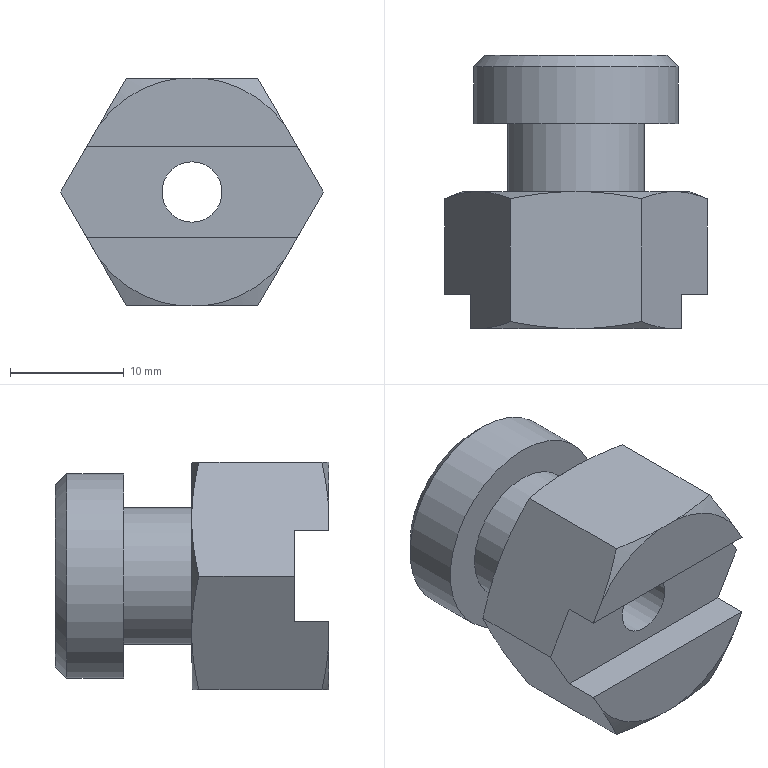Part | NX | 1 solid | 34 faces | box 23.094 x 24 x 20 mm | volume 5135 mm3 | plane 15 | cone 15 | cylinder 4 | commonest cylinder face diameters 5.3 x1 9 x1 12 x1 18 x1
STEP:
#1=CARTESIAN_POINT('',(9.238,-11.992,4.));
#2=VERTEX_POINT('',#1);
#3=CARTESIAN_POINT('',(9.146,-12.,4.159));
#4=VERTEX_POINT('',#3);
#5=CARTESIAN_POINT('',(9.238,-11.992,4.));
#6=CARTESIAN_POINT('',(9.207,-11.995,4.053));
#7=CARTESIAN_POINT('',(9.176,-11.998,4.106));
#8=CARTESIAN_POINT('',(9.146,-12.,4.159));
#9=B_SPLINE_CURVE_WITH_KNOTS('',3,(#5,#6,#7,#8),.UNSPECIFIED.,.F.,.F.,(4,4),(0.01293,0.01311),.UNSPECIFIED.);
#10=EDGE_CURVE('',#2,#4,#9,.T.);
#11=ORIENTED_EDGE('',*,*,#10,.F.);
#12=CARTESIAN_POINT('',(9.238,-9.,4.));
#13=VERTEX_POINT('',#12);
#14=CARTESIAN_POINT('',(9.238,12.,4.));
#15=DIRECTION('',(0.,1.,0.));
#16=VECTOR('',#15,1000.);
#17=LINE('',#14,#16);
#18=EDGE_CURVE('',#2,#13,#17,.T.);
#19=ORIENTED_EDGE('',*,*,#18,.T.);
#20=CARTESIAN_POINT('',(11.547,-9.,0.));
#21=VERTEX_POINT('',#20);
#22=CARTESIAN_POINT('',(5.774,-9.,10.));
#23=DIRECTION('',(0.5,0.,-0.866));
#24=VECTOR('',#23,1000.);
#25=LINE('',#22,#24);
#26=EDGE_CURVE('',#13,#21,#25,.T.);
#27=ORIENTED_EDGE('',*,*,#26,.T.);
#28=CARTESIAN_POINT('',(11.547,-0.6,0.));
#29=VERTEX_POINT('',#28);
#30=CARTESIAN_POINT('',(11.547,12.,0.));
#31=DIRECTION('',(0.,-1.,0.));
#32=VECTOR('',#31,1000.);
#33=LINE('',#30,#32);
#34=EDGE_CURVE('',#29,#21,#33,.T.);
#35=ORIENTED_EDGE('',*,*,#34,.F.);
#36=CARTESIAN_POINT('',(9.146,0.,4.159));
#37=VERTEX_POINT('',#36);
#38=CARTESIAN_POINT('',(9.146,0.,4.159));
#39=CARTESIAN_POINT('',(9.959,-0.06289,2.75));
#40=CARTESIAN_POINT('',(10.758,-0.2842,1.367));
#41=CARTESIAN_POINT('',(11.547,-0.6,0.));
#42=B_SPLINE_CURVE_WITH_KNOTS('',3,(#38,#39,#40,#41),.UNSPECIFIED.,.F.,.F.,(4,4),(0.01504,0.01991),.UNSPECIFIED.);
#43=EDGE_CURVE('',#37,#29,#42,.T.);
#44=ORIENTED_EDGE('',*,*,#43,.F.);
#45=CARTESIAN_POINT('',(8.175,0.,5.841));
#46=VERTEX_POINT('',#45);
#47=CARTESIAN_POINT('',(5.774,0.,10.));
#48=DIRECTION('',(0.5,0.,-0.866));
#49=VECTOR('',#48,1000.);
#50=LINE('',#47,#49);
#51=EDGE_CURVE('',#46,#37,#50,.T.);
#52=ORIENTED_EDGE('',*,*,#51,.F.);
#53=CARTESIAN_POINT('',(5.774,-0.6,10.));
#54=VERTEX_POINT('',#53);
#55=CARTESIAN_POINT('',(5.774,-0.6,10.));
#56=CARTESIAN_POINT('',(6.562,-0.2848,8.635));
#57=CARTESIAN_POINT('',(7.36,-0.06302,7.253));
#58=CARTESIAN_POINT('',(8.175,0.,5.841));
#59=B_SPLINE_CURVE_WITH_KNOTS('',3,(#55,#56,#57,#58),.UNSPECIFIED.,.F.,.F.,(4,4),(0.008294,0.01311),.UNSPECIFIED.);
#60=EDGE_CURVE('',#54,#46,#59,.T.);
#61=ORIENTED_EDGE('',*,*,#60,.F.);
#62=CARTESIAN_POINT('',(5.774,-11.4,10.));
#63=VERTEX_POINT('',#62);
#64=CARTESIAN_POINT('',(5.774,12.,10.));
#65=DIRECTION('',(0.,-1.,0.));
#66=VECTOR('',#65,1000.);
#67=LINE('',#64,#66);
#68=EDGE_CURVE('',#54,#63,#67,.T.);
#69=ORIENTED_EDGE('',*,*,#68,.T.);
#70=CARTESIAN_POINT('',(8.175,-12.,5.841));
#71=VERTEX_POINT('',#70);
#72=CARTESIAN_POINT('',(8.175,-12.,5.841));
#73=CARTESIAN_POINT('',(7.361,-11.937,7.25));
#74=CARTESIAN_POINT('',(6.563,-11.716,8.633));
#75=CARTESIAN_POINT('',(5.774,-11.4,10.));
#76=B_SPLINE_CURVE_WITH_KNOTS('',3,(#72,#73,#74,#75),.UNSPECIFIED.,.F.,.F.,(4,4),(0.01504,0.01991),.UNSPECIFIED.);
#77=EDGE_CURVE('',#71,#63,#76,.T.);
#78=ORIENTED_EDGE('',*,*,#77,.F.);
#79=CARTESIAN_POINT('',(5.774,-12.,10.));
#80=DIRECTION('',(0.5,0.,-0.866));
#81=VECTOR('',#80,1000.);
#82=LINE('',#79,#81);
#83=EDGE_CURVE('',#71,#4,#82,.T.);
#84=ORIENTED_EDGE('',*,*,#83,.T.);
#85=EDGE_LOOP('',(#11,#19,#27,#35,#44,#52,#61,#69,#78,#84));
#86=FACE_BOUND('',#85,.T.);
#87=CARTESIAN_POINT('',(5.774,12.,10.));
#88=DIRECTION('',(-0.866,0.,-0.5));
#89=DIRECTION('',(-0.5,0.,0.866));
#90=AXIS2_PLACEMENT_3D('',#87,#88,#89);
#91=PLANE('',#90);
#92=ADVANCED_FACE('',(#86),#91,.F.);
#93=CARTESIAN_POINT('',(5.774,-11.4,-10.));
#94=VERTEX_POINT('',#93);
#95=CARTESIAN_POINT('',(8.175,-12.,-5.841));
#96=VERTEX_POINT('',#95);
#97=CARTESIAN_POINT('',(5.774,-11.4,-10.));
#98=CARTESIAN_POINT('',(6.562,-11.715,-8.635));
#99=CARTESIAN_POINT('',(7.36,-11.937,-7.253));
#100=CARTESIAN_POINT('',(8.175,-12.,-5.841));
#101=B_SPLINE_CURVE_WITH_KNOTS('',3,(#97,#98,#99,#100),.UNSPECIFIED.,.F.,.F.,(4,4),(0.008294,0.01311),.UNSPECIFIED.);
#102=EDGE_CURVE('',#94,#96,#101,.T.);
#103=ORIENTED_EDGE('',*,*,#102,.F.);
#104=CARTESIAN_POINT('',(5.774,-0.6,-10.));
#105=VERTEX_POINT('',#104);
#106=CARTESIAN_POINT('',(5.774,12.,-10.));
#107=DIRECTION('',(0.,-1.,0.));
#108=VECTOR('',#107,1000.);
#109=LINE('',#106,#108);
#110=EDGE_CURVE('',#105,#94,#109,.T.);
#111=ORIENTED_EDGE('',*,*,#110,.F.);
#112=CARTESIAN_POINT('',(8.175,0.,-5.841));
#113=VERTEX_POINT('',#112);
#114=CARTESIAN_POINT('',(8.175,0.,-5.841));
#115=CARTESIAN_POINT('',(7.361,-0.06289,-7.25));
#116=CARTESIAN_POINT('',(6.563,-0.2842,-8.633));
#117=CARTESIAN_POINT('',(5.774,-0.6,-10.));
#118=B_SPLINE_CURVE_WITH_KNOTS('',3,(#114,#115,#116,#117),.UNSPECIFIED.,.F.,.F.,(4,4),(0.01504,0.01991),.UNSPECIFIED.);
#119=EDGE_CURVE('',#113,#105,#118,.T.);
#120=ORIENTED_EDGE('',*,*,#119,.F.);
#121=CARTESIAN_POINT('',(9.146,0.,-4.159));
#122=VERTEX_POINT('',#121);
#123=CARTESIAN_POINT('',(11.547,0.,0.));
#124=DIRECTION('',(-0.5,0.,-0.866));
#125=VECTOR('',#124,1000.);
#126=LINE('',#123,#125);
#127=EDGE_CURVE('',#122,#113,#126,.T.);
#128=ORIENTED_EDGE('',*,*,#127,.F.);
#129=CARTESIAN_POINT('',(11.547,-0.6,0.));
#130=CARTESIAN_POINT('',(10.759,-0.2848,-1.365));
#131=CARTESIAN_POINT('',(9.961,-0.06302,-2.747));
#132=CARTESIAN_POINT('',(9.146,0.,-4.159));
#133=B_SPLINE_CURVE_WITH_KNOTS('',3,(#129,#130,#131,#132),.UNSPECIFIED.,.F.,.F.,(4,4),(0.008294,0.01311),.UNSPECIFIED.);
#134=EDGE_CURVE('',#29,#122,#133,.T.);
#135=ORIENTED_EDGE('',*,*,#134,.F.);
#136=ORIENTED_EDGE('',*,*,#34,.T.);
#137=CARTESIAN_POINT('',(9.238,-9.,-4.));
#138=VERTEX_POINT('',#137);
#139=CARTESIAN_POINT('',(11.547,-9.,0.));
#140=DIRECTION('',(-0.5,0.,-0.866));
#141=VECTOR('',#140,1000.);
#142=LINE('',#139,#141);
#143=EDGE_CURVE('',#21,#138,#142,.T.);
#144=ORIENTED_EDGE('',*,*,#143,.T.);
#145=CARTESIAN_POINT('',(9.238,-11.992,-4.));
#146=VERTEX_POINT('',#145);
#147=CARTESIAN_POINT('',(9.238,12.,-4.));
#148=DIRECTION('',(0.,-1.,0.));
#149=VECTOR('',#148,1000.);
#150=LINE('',#147,#149);
#151=EDGE_CURVE('',#138,#146,#150,.T.);
#152=ORIENTED_EDGE('',*,*,#151,.T.);
#153=CARTESIAN_POINT('',(9.146,-12.,-4.159));
#154=VERTEX_POINT('',#153);
#155=CARTESIAN_POINT('',(9.146,-12.,-4.159));
#156=CARTESIAN_POINT('',(9.176,-11.998,-4.106));
#157=CARTESIAN_POINT('',(9.207,-11.995,-4.053));
#158=CARTESIAN_POINT('',(9.238,-11.992,-4.));
#159=B_SPLINE_CURVE_WITH_KNOTS('',3,(#155,#156,#157,#158),.UNSPECIFIED.,.F.,.F.,(4,4),(0.01504,0.01522),.UNSPECIFIED.);
#160=EDGE_CURVE('',#154,#146,#159,.T.);
#161=ORIENTED_EDGE('',*,*,#160,.F.);
#162=CARTESIAN_POINT('',(11.547,-12.,0.));
#163=DIRECTION('',(-0.5,0.,-0.866));
#164=VECTOR('',#163,1000.);
#165=LINE('',#162,#164);
#166=EDGE_CURVE('',#154,#96,#165,.T.);
#167=ORIENTED_EDGE('',*,*,#166,.T.);
#168=EDGE_LOOP('',(#103,#111,#120,#128,#135,#136,#144,#152,#161,#167));
#169=FACE_BOUND('',#168,.T.);
#170=CARTESIAN_POINT('',(11.547,12.,0.));
#171=DIRECTION('',(-0.866,0.,0.5));
#172=DIRECTION('',(0.5,0.,0.866));
#173=AXIS2_PLACEMENT_3D('',#170,#171,#172);
#174=PLANE('',#173);
#175=ADVANCED_FACE('',(#169),#174,.F.);
#176=CARTESIAN_POINT('',(-5.774,-11.4,-10.));
#177=VERTEX_POINT('',#176);
#178=CARTESIAN_POINT('',(-0.9707,-12.,-10.));
#179=VERTEX_POINT('',#178);
#180=CARTESIAN_POINT('',(-5.774,-11.4,-10.));
#181=CARTESIAN_POINT('',(-4.196,-11.716,-10.));
#182=CARTESIAN_POINT('',(-2.599,-11.937,-10.));
#183=CARTESIAN_POINT('',(-0.9707,-12.,-10.));
#184=B_SPLINE_CURVE_WITH_KNOTS('',3,(#180,#181,#182,#183),.UNSPECIFIED.,.F.,.F.,(4,4),(0.007166,0.01199),.UNSPECIFIED.);
#185=EDGE_CURVE('',#177,#179,#184,.T.);
#186=ORIENTED_EDGE('',*,*,#185,.F.);
#187=CARTESIAN_POINT('',(-5.774,-0.6,-10.));
#188=VERTEX_POINT('',#187);
#189=CARTESIAN_POINT('',(-5.774,12.,-10.));
#190=DIRECTION('',(0.,-1.,0.));
#191=VECTOR('',#190,1000.);
#192=LINE('',#189,#191);
#193=EDGE_CURVE('',#188,#177,#192,.T.);
#194=ORIENTED_EDGE('',*,*,#193,.F.);
#195=CARTESIAN_POINT('',(-0.9707,0.,-10.));
#196=VERTEX_POINT('',#195);
#197=CARTESIAN_POINT('',(-0.9707,0.,-10.));
#198=CARTESIAN_POINT('',(-2.598,-0.06287,-10.));
#199=CARTESIAN_POINT('',(-4.194,-0.2842,-10.));
#200=CARTESIAN_POINT('',(-5.774,-0.6,-10.));
#201=B_SPLINE_CURVE_WITH_KNOTS('',3,(#197,#198,#199,#200),.UNSPECIFIED.,.F.,.F.,(4,4),(0.01391,0.01876),.UNSPECIFIED.);
#202=EDGE_CURVE('',#196,#188,#201,.T.);
#203=ORIENTED_EDGE('',*,*,#202,.F.);
#204=CARTESIAN_POINT('',(0.9707,0.,-10.));
#205=VERTEX_POINT('',#204);
#206=CARTESIAN_POINT('',(5.774,0.,-10.));
#207=DIRECTION('',(-1.,0.,0.));
#208=VECTOR('',#207,1000.);
#209=LINE('',#206,#208);
#210=EDGE_CURVE('',#205,#196,#209,.T.);
#211=ORIENTED_EDGE('',*,*,#210,.F.);
#212=CARTESIAN_POINT('',(5.774,-0.6,-10.));
#213=CARTESIAN_POINT('',(4.196,-0.2844,-10.));
#214=CARTESIAN_POINT('',(2.599,-0.06293,-10.));
#215=CARTESIAN_POINT('',(0.9707,0.,-10.));
#216=B_SPLINE_CURVE_WITH_KNOTS('',3,(#212,#213,#214,#215),.UNSPECIFIED.,.F.,.F.,(4,4),(0.007166,0.01199),.UNSPECIFIED.);
#217=EDGE_CURVE('',#105,#205,#216,.T.);
#218=ORIENTED_EDGE('',*,*,#217,.F.);
#219=ORIENTED_EDGE('',*,*,#110,.T.);
#220=CARTESIAN_POINT('',(0.9707,-12.,-10.));
#221=VERTEX_POINT('',#220);
#222=CARTESIAN_POINT('',(0.9707,-12.,-10.));
#223=CARTESIAN_POINT('',(2.598,-11.937,-10.));
#224=CARTESIAN_POINT('',(4.194,-11.716,-10.));
#225=CARTESIAN_POINT('',(5.774,-11.4,-10.));
#226=B_SPLINE_CURVE_WITH_KNOTS('',3,(#222,#223,#224,#225),.UNSPECIFIED.,.F.,.F.,(4,4),(0.01391,0.01876),.UNSPECIFIED.);
#227=EDGE_CURVE('',#221,#94,#226,.T.);
#228=ORIENTED_EDGE('',*,*,#227,.F.);
#229=CARTESIAN_POINT('',(5.774,-12.,-10.));
#230=DIRECTION('',(-1.,0.,0.));
#231=VECTOR('',#230,1000.);
#232=LINE('',#229,#231);
#233=EDGE_CURVE('',#221,#179,#232,.T.);
#234=ORIENTED_EDGE('',*,*,#233,.T.);
#235=EDGE_LOOP('',(#186,#194,#203,#211,#218,#219,#228,#234));
#236=FACE_BOUND('',#235,.T.);
#237=CARTESIAN_POINT('',(5.774,12.,-10.));
#238=DIRECTION('',(0.,0.,1.));
#239=DIRECTION('',(1.,0.,0.));
#240=AXIS2_PLACEMENT_3D('',#237,#238,#239);
#241=PLANE('',#240);
#242=ADVANCED_FACE('',(#236),#241,.F.);
#243=CARTESIAN_POINT('',(-9.238,-11.992,-4.));
#244=VERTEX_POINT('',#243);
#245=CARTESIAN_POINT('',(-9.146,-12.,-4.159));
#246=VERTEX_POINT('',#245);
#247=CARTESIAN_POINT('',(-9.238,-11.992,-4.));
#248=CARTESIAN_POINT('',(-9.207,-11.995,-4.053));
#249=CARTESIAN_POINT('',(-9.176,-11.998,-4.106));
#250=CARTESIAN_POINT('',(-9.146,-12.,-4.159));
#251=B_SPLINE_CURVE_WITH_KNOTS('',3,(#247,#248,#249,#250),.UNSPECIFIED.,.F.,.F.,(4,4),(0.01293,0.01311),.UNSPECIFIED.);
#252=EDGE_CURVE('',#244,#246,#251,.T.);
#253=ORIENTED_EDGE('',*,*,#252,.F.);
#254=CARTESIAN_POINT('',(-9.238,-9.,-4.));
#255=VERTEX_POINT('',#254);
#256=CARTESIAN_POINT('',(-9.238,12.,-4.));
#257=DIRECTION('',(0.,1.,0.));
#258=VECTOR('',#257,1000.);
#259=LINE('',#256,#258);
#260=EDGE_CURVE('',#244,#255,#259,.T.);
#261=ORIENTED_EDGE('',*,*,#260,.T.);
#262=CARTESIAN_POINT('',(-11.547,-9.,0.));
#263=VERTEX_POINT('',#262);
#264=CARTESIAN_POINT('',(-5.774,-9.,-10.));
#265=DIRECTION('',(-0.5,0.,0.866));
#266=VECTOR('',#265,1000.);
#267=LINE('',#264,#266);
#268=EDGE_CURVE('',#255,#263,#267,.T.);
#269=ORIENTED_EDGE('',*,*,#268,.T.);
#270=CARTESIAN_POINT('',(-11.547,-0.6,0.));
#271=VERTEX_POINT('',#270);
#272=CARTESIAN_POINT('',(-11.547,12.,0.));
#273=DIRECTION('',(0.,-1.,0.));
#274=VECTOR('',#273,1000.);
#275=LINE('',#272,#274);
#276=EDGE_CURVE('',#271,#263,#275,.T.);
#277=ORIENTED_EDGE('',*,*,#276,.F.);
#278=CARTESIAN_POINT('',(-9.146,0.,-4.159));
#279=VERTEX_POINT('',#278);
#280=CARTESIAN_POINT('',(-9.146,0.,-4.159));
#281=CARTESIAN_POINT('',(-9.959,-0.06289,-2.75));
#282=CARTESIAN_POINT('',(-10.758,-0.2842,-1.367));
#283=CARTESIAN_POINT('',(-11.547,-0.6,0.));
#284=B_SPLINE_CURVE_WITH_KNOTS('',3,(#280,#281,#282,#283),.UNSPECIFIED.,.F.,.F.,(4,4),(0.01504,0.01991),.UNSPECIFIED.);
#285=EDGE_CURVE('',#279,#271,#284,.T.);
#286=ORIENTED_EDGE('',*,*,#285,.F.);
#287=CARTESIAN_POINT('',(-8.175,0.,-5.841));
#288=VERTEX_POINT('',#287);
#289=CARTESIAN_POINT('',(-5.774,0.,-10.));
#290=DIRECTION('',(-0.5,0.,0.866));
#291=VECTOR('',#290,1000.);
#292=LINE('',#289,#291);
#293=EDGE_CURVE('',#288,#279,#292,.T.);
#294=ORIENTED_EDGE('',*,*,#293,.F.);
#295=CARTESIAN_POINT('',(-5.774,-0.6,-10.));
#296=CARTESIAN_POINT('',(-6.562,-0.2848,-8.635));
#297=CARTESIAN_POINT('',(-7.36,-0.06302,-7.253));
#298=CARTESIAN_POINT('',(-8.175,0.,-5.841));
#299=B_SPLINE_CURVE_WITH_KNOTS('',3,(#295,#296,#297,#298),.UNSPECIFIED.,.F.,.F.,(4,4),(0.008294,0.01311),.UNSPECIFIED.);
#300=EDGE_CURVE('',#188,#288,#299,.T.);
#301=ORIENTED_EDGE('',*,*,#300,.F.);
#302=ORIENTED_EDGE('',*,*,#193,.T.);
#303=CARTESIAN_POINT('',(-8.175,-12.,-5.841));
#304=VERTEX_POINT('',#303);
#305=CARTESIAN_POINT('',(-8.175,-12.,-5.841));
#306=CARTESIAN_POINT('',(-7.361,-11.937,-7.25));
#307=CARTESIAN_POINT('',(-6.563,-11.716,-8.633));
#308=CARTESIAN_POINT('',(-5.774,-11.4,-10.));
#309=B_SPLINE_CURVE_WITH_KNOTS('',3,(#305,#306,#307,#308),.UNSPECIFIED.,.F.,.F.,(4,4),(0.01504,0.01991),.UNSPECIFIED.);
#310=EDGE_CURVE('',#304,#177,#309,.T.);
#311=ORIENTED_EDGE('',*,*,#310,.F.);
#312=CARTESIAN_POINT('',(-5.774,-12.,-10.));
#313=DIRECTION('',(-0.5,0.,0.866));
#314=VECTOR('',#313,1000.);
#315=LINE('',#312,#314);
#316=EDGE_CURVE('',#304,#246,#315,.T.);
#317=ORIENTED_EDGE('',*,*,#316,.T.);
#318=EDGE_LOOP('',(#253,#261,#269,#277,#286,#294,#301,#302,#311,#317));
#319=FACE_BOUND('',#318,.T.);
#320=CARTESIAN_POINT('',(-5.774,12.,-10.));
#321=DIRECTION('',(0.866,0.,0.5));
#322=DIRECTION('',(0.5,0.,-0.866));
#323=AXIS2_PLACEMENT_3D('',#320,#321,#322);
#324=PLANE('',#323);
#325=ADVANCED_FACE('',(#319),#324,.F.);
#326=CARTESIAN_POINT('',(-5.774,-11.4,10.));
#327=VERTEX_POINT('',#326);
#328=CARTESIAN_POINT('',(-8.175,-12.,5.841));
#329=VERTEX_POINT('',#328);
#330=CARTESIAN_POINT('',(-5.774,-11.4,10.));
#331=CARTESIAN_POINT('',(-6.562,-11.715,8.635));
#332=CARTESIAN_POINT('',(-7.36,-11.937,7.253));
#333=CARTESIAN_POINT('',(-8.175,-12.,5.841));
#334=B_SPLINE_CURVE_WITH_KNOTS('',3,(#330,#331,#332,#333),.UNSPECIFIED.,.F.,.F.,(4,4),(0.008294,0.01311),.UNSPECIFIED.);
#335=EDGE_CURVE('',#327,#329,#334,.T.);
#336=ORIENTED_EDGE('',*,*,#335,.F.);
#337=CARTESIAN_POINT('',(-5.774,-0.6,10.));
#338=VERTEX_POINT('',#337);
#339=CARTESIAN_POINT('',(-5.774,12.,10.));
#340=DIRECTION('',(0.,-1.,0.));
#341=VECTOR('',#340,1000.);
#342=LINE('',#339,#341);
#343=EDGE_CURVE('',#338,#327,#342,.T.);
#344=ORIENTED_EDGE('',*,*,#343,.F.);
#345=CARTESIAN_POINT('',(-8.175,0.,5.841));
#346=VERTEX_POINT('',#345);
#347=CARTESIAN_POINT('',(-8.175,0.,5.841));
#348=CARTESIAN_POINT('',(-7.361,-0.06289,7.25));
#349=CARTESIAN_POINT('',(-6.563,-0.2842,8.633));
#350=CARTESIAN_POINT('',(-5.774,-0.6,10.));
#351=B_SPLINE_CURVE_WITH_KNOTS('',3,(#347,#348,#349,#350),.UNSPECIFIED.,.F.,.F.,(4,4),(0.01504,0.01991),.UNSPECIFIED.);
#352=EDGE_CURVE('',#346,#338,#351,.T.);
#353=ORIENTED_EDGE('',*,*,#352,.F.);
#354=CARTESIAN_POINT('',(-9.146,0.,4.159));
#355=VERTEX_POINT('',#354);
#356=CARTESIAN_POINT('',(-11.547,0.,0.));
#357=DIRECTION('',(0.5,0.,0.866));
#358=VECTOR('',#357,1000.);
#359=LINE('',#356,#358);
#360=EDGE_CURVE('',#355,#346,#359,.T.);
#361=ORIENTED_EDGE('',*,*,#360,.F.);
#362=CARTESIAN_POINT('',(-11.547,-0.6,0.));
#363=CARTESIAN_POINT('',(-10.759,-0.2848,1.365));
#364=CARTESIAN_POINT('',(-9.961,-0.06302,2.747));
#365=CARTESIAN_POINT('',(-9.146,0.,4.159));
#366=B_SPLINE_CURVE_WITH_KNOTS('',3,(#362,#363,#364,#365),.UNSPECIFIED.,.F.,.F.,(4,4),(0.008294,0.01311),.UNSPECIFIED.);
#367=EDGE_CURVE('',#271,#355,#366,.T.);
#368=ORIENTED_EDGE('',*,*,#367,.F.);
#369=ORIENTED_EDGE('',*,*,#276,.T.);
#370=CARTESIAN_POINT('',(-9.238,-9.,4.));
#371=VERTEX_POINT('',#370);
#372=CARTESIAN_POINT('',(-11.547,-9.,0.));
#373=DIRECTION('',(0.5,0.,0.866));
#374=VECTOR('',#373,1000.);
#375=LINE('',#372,#374);
#376=EDGE_CURVE('',#263,#371,#375,.T.);
#377=ORIENTED_EDGE('',*,*,#376,.T.);
#378=CARTESIAN_POINT('',(-9.238,-11.992,4.));
#379=VERTEX_POINT('',#378);
#380=CARTESIAN_POINT('',(-9.238,12.,4.));
#381=DIRECTION('',(0.,-1.,0.));
#382=VECTOR('',#381,1000.);
#383=LINE('',#380,#382);
#384=EDGE_CURVE('',#371,#379,#383,.T.);
#385=ORIENTED_EDGE('',*,*,#384,.T.);
#386=CARTESIAN_POINT('',(-9.146,-12.,4.159));
#387=VERTEX_POINT('',#386);
#388=CARTESIAN_POINT('',(-9.146,-12.,4.159));
#389=CARTESIAN_POINT('',(-9.176,-11.998,4.106));
#390=CARTESIAN_POINT('',(-9.207,-11.995,4.053));
#391=CARTESIAN_POINT('',(-9.238,-11.992,4.));
#392=B_SPLINE_CURVE_WITH_KNOTS('',3,(#388,#389,#390,#391),.UNSPECIFIED.,.F.,.F.,(4,4),(0.01504,0.01522),.UNSPECIFIED.);
#393=EDGE_CURVE('',#387,#379,#392,.T.);
#394=ORIENTED_EDGE('',*,*,#393,.F.);
#395=CARTESIAN_POINT('',(-11.547,-12.,0.));
#396=DIRECTION('',(0.5,0.,0.866));
#397=VECTOR('',#396,1000.);
#398=LINE('',#395,#397);
#399=EDGE_CURVE('',#387,#329,#398,.T.);
#400=ORIENTED_EDGE('',*,*,#399,.T.);
#401=EDGE_LOOP('',(#336,#344,#353,#361,#368,#369,#377,#385,#394,#400));
#402=FACE_BOUND('',#401,.T.);
#403=CARTESIAN_POINT('',(-11.547,12.,0.));
#404=DIRECTION('',(0.866,0.,-0.5));
#405=DIRECTION('',(-0.5,0.,-0.866));
#406=AXIS2_PLACEMENT_3D('',#403,#404,#405);
#407=PLANE('',#406);
#408=ADVANCED_FACE('',(#402),#407,.F.);
#409=CARTESIAN_POINT('',(0.9707,-12.,10.));
#410=VERTEX_POINT('',#409);
#411=CARTESIAN_POINT('',(5.774,-11.4,10.));
#412=CARTESIAN_POINT('',(4.196,-11.716,10.));
#413=CARTESIAN_POINT('',(2.599,-11.937,10.));
#414=CARTESIAN_POINT('',(0.9707,-12.,10.));
#415=B_SPLINE_CURVE_WITH_KNOTS('',3,(#411,#412,#413,#414),.UNSPECIFIED.,.F.,.F.,(4,4),(0.007166,0.01199),.UNSPECIFIED.);
#416=EDGE_CURVE('',#63,#410,#415,.T.);
#417=ORIENTED_EDGE('',*,*,#416,.F.);
#418=ORIENTED_EDGE('',*,*,#68,.F.);
#419=CARTESIAN_POINT('',(0.9707,0.,10.));
#420=VERTEX_POINT('',#419);
#421=CARTESIAN_POINT('',(0.9707,0.,10.));
#422=CARTESIAN_POINT('',(2.598,-0.06287,10.));
#423=CARTESIAN_POINT('',(4.194,-0.2842,10.));
#424=CARTESIAN_POINT('',(5.774,-0.6,10.));
#425=B_SPLINE_CURVE_WITH_KNOTS('',3,(#421,#422,#423,#424),.UNSPECIFIED.,.F.,.F.,(4,4),(0.01391,0.01876),.UNSPECIFIED.);
#426=EDGE_CURVE('',#420,#54,#425,.T.);
#427=ORIENTED_EDGE('',*,*,#426,.F.);
#428=CARTESIAN_POINT('',(-0.9707,0.,10.));
#429=VERTEX_POINT('',#428);
#430=CARTESIAN_POINT('',(-5.774,0.,10.));
#431=DIRECTION('',(1.,0.,0.));
#432=VECTOR('',#431,1000.);
#433=LINE('',#430,#432);
#434=EDGE_CURVE('',#429,#420,#433,.T.);
#435=ORIENTED_EDGE('',*,*,#434,.F.);
#436=CARTESIAN_POINT('',(-5.774,-0.6,10.));
#437=CARTESIAN_POINT('',(-4.196,-0.2844,10.));
#438=CARTESIAN_POINT('',(-2.599,-0.06293,10.));
#439=CARTESIAN_POINT('',(-0.9707,0.,10.));
#440=B_SPLINE_CURVE_WITH_KNOTS('',3,(#436,#437,#438,#439),.UNSPECIFIED.,.F.,.F.,(4,4),(0.007166,0.01199),.UNSPECIFIED.);
#441=EDGE_CURVE('',#338,#429,#440,.T.);
#442=ORIENTED_EDGE('',*,*,#441,.F.);
#443=ORIENTED_EDGE('',*,*,#343,.T.);
#444=CARTESIAN_POINT('',(-0.9707,-12.,10.));
#445=VERTEX_POINT('',#444);
#446=CARTESIAN_POINT('',(-0.9707,-12.,10.));
#447=CARTESIAN_POINT('',(-2.598,-11.937,10.));
#448=CARTESIAN_POINT('',(-4.194,-11.716,10.));
#449=CARTESIAN_POINT('',(-5.774,-11.4,10.));
#450=B_SPLINE_CURVE_WITH_KNOTS('',3,(#446,#447,#448,#449),.UNSPECIFIED.,.F.,.F.,(4,4),(0.01391,0.01876),.UNSPECIFIED.);
#451=EDGE_CURVE('',#445,#327,#450,.T.);
#452=ORIENTED_EDGE('',*,*,#451,.F.);
#453=CARTESIAN_POINT('',(-5.774,-12.,10.));
#454=DIRECTION('',(1.,0.,0.));
#455=VECTOR('',#454,1000.);
#456=LINE('',#453,#455);
#457=EDGE_CURVE('',#445,#410,#456,.T.);
#458=ORIENTED_EDGE('',*,*,#457,.T.);
#459=EDGE_LOOP('',(#417,#418,#427,#435,#442,#443,#452,#458));
#460=FACE_BOUND('',#459,.T.);
#461=CARTESIAN_POINT('',(-5.774,12.,10.));
#462=DIRECTION('',(0.,0.,-1.));
#463=DIRECTION('',(-1.,0.,0.));
#464=AXIS2_PLACEMENT_3D('',#461,#462,#463);
#465=PLANE('',#464);
#466=ADVANCED_FACE('',(#460),#465,.F.);
#467=CARTESIAN_POINT('',(0.,-12.,0.));
#468=DIRECTION('',(0.,1.,0.));
#469=DIRECTION('',(0.,0.,1.));
#470=AXIS2_PLACEMENT_3D('',#467,#468,#469);
#471=CIRCLE('',#470,10.047);
#472=EDGE_CURVE('',#410,#71,#471,.T.);
#473=ORIENTED_EDGE('',*,*,#472,.F.);
#474=ORIENTED_EDGE('',*,*,#457,.F.);
#475=CARTESIAN_POINT('',(0.,-12.,0.));
#476=DIRECTION('',(0.,1.,0.));
#477=DIRECTION('',(0.,0.,1.));
#478=AXIS2_PLACEMENT_3D('',#475,#476,#477);
#479=CIRCLE('',#478,10.047);
#480=EDGE_CURVE('',#329,#445,#479,.T.);
#481=ORIENTED_EDGE('',*,*,#480,.F.);
#482=ORIENTED_EDGE('',*,*,#399,.F.);
#483=CARTESIAN_POINT('',(-9.216,-12.,4.));
#484=VERTEX_POINT('',#483);
#485=CARTESIAN_POINT('',(0.,-12.,0.));
#486=DIRECTION('',(0.,1.,0.));
#487=DIRECTION('',(0.,0.,1.));
#488=AXIS2_PLACEMENT_3D('',#485,#486,#487);
#489=CIRCLE('',#488,10.047);
#490=EDGE_CURVE('',#484,#387,#489,.T.);
#491=ORIENTED_EDGE('',*,*,#490,.F.);
#492=CARTESIAN_POINT('',(9.216,-12.,4.));
#493=VERTEX_POINT('',#492);
#494=CARTESIAN_POINT('',(0.,-12.,4.));
#495=DIRECTION('',(1.,0.,0.));
#496=VECTOR('',#495,1000.);
#497=LINE('',#494,#496);
#498=EDGE_CURVE('',#484,#493,#497,.T.);
#499=ORIENTED_EDGE('',*,*,#498,.T.);
#500=CARTESIAN_POINT('',(0.,-12.,0.));
#501=DIRECTION('',(0.,1.,0.));
#502=DIRECTION('',(0.,0.,1.));
#503=AXIS2_PLACEMENT_3D('',#500,#501,#502);
#504=CIRCLE('',#503,10.047);
#505=EDGE_CURVE('',#4,#493,#504,.T.);
#506=ORIENTED_EDGE('',*,*,#505,.F.);
#507=ORIENTED_EDGE('',*,*,#83,.F.);
#508=EDGE_LOOP('',(#473,#474,#481,#482,#491,#499,#506,#507));
#509=FACE_BOUND('',#508,.T.);
#510=CARTESIAN_POINT('',(0.,-12.,0.));
#511=DIRECTION('',(0.,1.,0.));
#512=DIRECTION('',(0.,0.,1.));
#513=AXIS2_PLACEMENT_3D('',#510,#511,#512);
#514=PLANE('',#513);
#515=ADVANCED_FACE('',(#509),#514,.F.);
#516=CARTESIAN_POINT('',(9.216,-12.,-4.));
#517=VERTEX_POINT('',#516);
#518=CARTESIAN_POINT('',(0.,-12.,0.));
#519=DIRECTION('',(0.,1.,0.));
#520=DIRECTION('',(0.,0.,1.));
#521=AXIS2_PLACEMENT_3D('',#518,#519,#520);
#522=CIRCLE('',#521,10.047);
#523=EDGE_CURVE('',#517,#154,#522,.T.);
#524=ORIENTED_EDGE('',*,*,#523,.F.);
#525=CARTESIAN_POINT('',(-9.216,-12.,-4.));
#526=VERTEX_POINT('',#525);
#527=CARTESIAN_POINT('',(0.,-12.,-4.));
#528=DIRECTION('',(-1.,0.,0.));
#529=VECTOR('',#528,1000.);
#530=LINE('',#527,#529);
#531=EDGE_CURVE('',#517,#526,#530,.T.);
#532=ORIENTED_EDGE('',*,*,#531,.T.);
#533=CARTESIAN_POINT('',(0.,-12.,0.));
#534=DIRECTION('',(0.,1.,0.));
#535=DIRECTION('',(0.,0.,1.));
#536=AXIS2_PLACEMENT_3D('',#533,#534,#535);
#537=CIRCLE('',#536,10.047);
#538=EDGE_CURVE('',#246,#526,#537,.T.);
#539=ORIENTED_EDGE('',*,*,#538,.F.);
#540=ORIENTED_EDGE('',*,*,#316,.F.);
#541=CARTESIAN_POINT('',(0.,-12.,0.));
#542=DIRECTION('',(0.,1.,0.));
#543=DIRECTION('',(0.,0.,1.));
#544=AXIS2_PLACEMENT_3D('',#541,#542,#543);
#545=CIRCLE('',#544,10.047);
#546=EDGE_CURVE('',#179,#304,#545,.T.);
#547=ORIENTED_EDGE('',*,*,#546,.F.);
#548=ORIENTED_EDGE('',*,*,#233,.F.);
#549=CARTESIAN_POINT('',(0.,-12.,0.));
#550=DIRECTION('',(0.,1.,0.));
#551=DIRECTION('',(0.,0.,1.));
#552=AXIS2_PLACEMENT_3D('',#549,#550,#551);
#553=CIRCLE('',#552,10.047);
#554=EDGE_CURVE('',#96,#221,#553,.T.);
#555=ORIENTED_EDGE('',*,*,#554,.F.);
#556=ORIENTED_EDGE('',*,*,#166,.F.);
#557=EDGE_LOOP('',(#524,#532,#539,#540,#547,#548,#555,#556));
#558=FACE_BOUND('',#557,.T.);
#559=CARTESIAN_POINT('',(0.,-12.,0.));
#560=DIRECTION('',(0.,1.,0.));
#561=DIRECTION('',(0.,0.,1.));
#562=AXIS2_PLACEMENT_3D('',#559,#560,#561);
#563=PLANE('',#562);
#564=ADVANCED_FACE('',(#558),#563,.F.);
#565=CARTESIAN_POINT('',(-9.238,-11.992,4.));
#566=CARTESIAN_POINT('',(-9.231,-11.995,4.));
#567=CARTESIAN_POINT('',(-9.223,-11.997,4.));
#568=CARTESIAN_POINT('',(-9.216,-12.,4.));
#569=B_SPLINE_CURVE_WITH_KNOTS('',3,(#565,#566,#567,#568),.UNSPECIFIED.,.F.,.F.,(4,4),(0.01188,0.0119),.UNSPECIFIED.);
#570=EDGE_CURVE('',#379,#484,#569,.T.);
#571=ORIENTED_EDGE('',*,*,#570,.F.);
#572=ORIENTED_EDGE('',*,*,#384,.F.);
#573=CARTESIAN_POINT('',(-15.,-9.,4.));
#574=DIRECTION('',(-1.,0.,0.));
#575=VECTOR('',#574,1000.);
#576=LINE('',#573,#575);
#577=EDGE_CURVE('',#13,#371,#576,.T.);
#578=ORIENTED_EDGE('',*,*,#577,.F.);
#579=ORIENTED_EDGE('',*,*,#18,.F.);
#580=CARTESIAN_POINT('',(9.216,-12.,4.));
#581=CARTESIAN_POINT('',(9.223,-11.997,4.));
#582=CARTESIAN_POINT('',(9.231,-11.995,4.));
#583=CARTESIAN_POINT('',(9.238,-11.992,4.));
#584=B_SPLINE_CURVE_WITH_KNOTS('',3,(#580,#581,#582,#583),.UNSPECIFIED.,.F.,.F.,(4,4),(0.03106,0.03109),.UNSPECIFIED.);
#585=EDGE_CURVE('',#493,#2,#584,.T.);
#586=ORIENTED_EDGE('',*,*,#585,.F.);
#587=ORIENTED_EDGE('',*,*,#498,.F.);
#588=EDGE_LOOP('',(#571,#572,#578,#579,#586,#587));
#589=FACE_BOUND('',#588,.T.);
#590=CARTESIAN_POINT('',(-15.,-9.,4.));
#591=DIRECTION('',(0.,0.,1.));
#592=DIRECTION('',(1.,0.,0.));
#593=AXIS2_PLACEMENT_3D('',#590,#591,#592);
#594=PLANE('',#593);
#595=ADVANCED_FACE('',(#589),#594,.F.);
#596=CARTESIAN_POINT('',(9.238,-11.992,-4.));
#597=CARTESIAN_POINT('',(9.231,-11.995,-4.));
#598=CARTESIAN_POINT('',(9.223,-11.997,-4.));
#599=CARTESIAN_POINT('',(9.216,-12.,-4.));
#600=B_SPLINE_CURVE_WITH_KNOTS('',3,(#596,#597,#598,#599),.UNSPECIFIED.,.F.,.F.,(4,4),(0.01188,0.0119),.UNSPECIFIED.);
#601=EDGE_CURVE('',#146,#517,#600,.T.);
#602=ORIENTED_EDGE('',*,*,#601,.F.);
#603=ORIENTED_EDGE('',*,*,#151,.F.);
#604=CARTESIAN_POINT('',(-15.,-9.,-4.));
#605=DIRECTION('',(1.,0.,0.));
#606=VECTOR('',#605,1000.);
#607=LINE('',#604,#606);
#608=EDGE_CURVE('',#255,#138,#607,.T.);
#609=ORIENTED_EDGE('',*,*,#608,.F.);
#610=ORIENTED_EDGE('',*,*,#260,.F.);
#611=CARTESIAN_POINT('',(-9.216,-12.,-4.));
#612=CARTESIAN_POINT('',(-9.223,-11.997,-4.));
#613=CARTESIAN_POINT('',(-9.231,-11.995,-4.));
#614=CARTESIAN_POINT('',(-9.238,-11.992,-4.));
#615=B_SPLINE_CURVE_WITH_KNOTS('',3,(#611,#612,#613,#614),.UNSPECIFIED.,.F.,.F.,(4,4),(0.03106,0.03109),.UNSPECIFIED.);
#616=EDGE_CURVE('',#526,#244,#615,.T.);
#617=ORIENTED_EDGE('',*,*,#616,.F.);
#618=ORIENTED_EDGE('',*,*,#531,.F.);
#619=EDGE_LOOP('',(#602,#603,#609,#610,#617,#618));
#620=FACE_BOUND('',#619,.T.);
#621=CARTESIAN_POINT('',(-15.,-9.,-4.));
#622=DIRECTION('',(0.,0.,-1.));
#623=DIRECTION('',(-1.,0.,0.));
#624=AXIS2_PLACEMENT_3D('',#621,#622,#623);
#625=PLANE('',#624);
#626=ADVANCED_FACE('',(#620),#625,.F.);
#627=CARTESIAN_POINT('',(0.,0.,6.));
#628=VERTEX_POINT('',#627);
#629=CARTESIAN_POINT('',(0.,0.,0.));
#630=DIRECTION('',(0.,1.,0.));
#631=DIRECTION('',(0.,0.,1.));
#632=AXIS2_PLACEMENT_3D('',#629,#630,#631);
#633=CIRCLE('',#632,6.);
#634=EDGE_CURVE('',#628,#628,#633,.T.);
#635=ORIENTED_EDGE('',*,*,#634,.F.);
#636=EDGE_LOOP('',(#635));
#637=FACE_BOUND('',#636,.T.);
#638=ORIENTED_EDGE('',*,*,#434,.T.);
#639=CARTESIAN_POINT('',(0.,0.,0.));
#640=DIRECTION('',(0.,1.,0.));
#641=DIRECTION('',(0.,0.,1.));
#642=AXIS2_PLACEMENT_3D('',#639,#640,#641);
#643=CIRCLE('',#642,10.047);
#644=EDGE_CURVE('',#420,#46,#643,.T.);
#645=ORIENTED_EDGE('',*,*,#644,.T.);
#646=ORIENTED_EDGE('',*,*,#51,.T.);
#647=CARTESIAN_POINT('',(0.,0.,0.));
#648=DIRECTION('',(0.,1.,0.));
#649=DIRECTION('',(0.,0.,1.));
#650=AXIS2_PLACEMENT_3D('',#647,#648,#649);
#651=CIRCLE('',#650,10.047);
#652=EDGE_CURVE('',#37,#122,#651,.T.);
#653=ORIENTED_EDGE('',*,*,#652,.T.);
#654=ORIENTED_EDGE('',*,*,#127,.T.);
#655=CARTESIAN_POINT('',(0.,0.,0.));
#656=DIRECTION('',(0.,1.,0.));
#657=DIRECTION('',(0.,0.,1.));
#658=AXIS2_PLACEMENT_3D('',#655,#656,#657);
#659=CIRCLE('',#658,10.047);
#660=EDGE_CURVE('',#113,#205,#659,.T.);
#661=ORIENTED_EDGE('',*,*,#660,.T.);
#662=ORIENTED_EDGE('',*,*,#210,.T.);
#663=CARTESIAN_POINT('',(0.,0.,0.));
#664=DIRECTION('',(0.,1.,0.));
#665=DIRECTION('',(0.,0.,1.));
#666=AXIS2_PLACEMENT_3D('',#663,#664,#665);
#667=CIRCLE('',#666,10.047);
#668=EDGE_CURVE('',#196,#288,#667,.T.);
#669=ORIENTED_EDGE('',*,*,#668,.T.);
#670=ORIENTED_EDGE('',*,*,#293,.T.);
#671=CARTESIAN_POINT('',(0.,0.,0.));
#672=DIRECTION('',(0.,1.,0.));
#673=DIRECTION('',(0.,0.,1.));
#674=AXIS2_PLACEMENT_3D('',#671,#672,#673);
#675=CIRCLE('',#674,10.047);
#676=EDGE_CURVE('',#279,#355,#675,.T.);
#677=ORIENTED_EDGE('',*,*,#676,.T.);
#678=ORIENTED_EDGE('',*,*,#360,.T.);
#679=CARTESIAN_POINT('',(0.,0.,0.));
#680=DIRECTION('',(0.,1.,0.));
#681=DIRECTION('',(0.,0.,1.));
#682=AXIS2_PLACEMENT_3D('',#679,#680,#681);
#683=CIRCLE('',#682,10.047);
#684=EDGE_CURVE('',#346,#429,#683,.T.);
#685=ORIENTED_EDGE('',*,*,#684,.T.);
#686=EDGE_LOOP('',(#638,#645,#646,#653,#654,#661,#662,#669,#670,#677,#678,#685));
#687=FACE_BOUND('',#686,.T.);
#688=CARTESIAN_POINT('',(0.,0.,0.));
#689=DIRECTION('',(0.,1.,0.));
#690=DIRECTION('',(0.,0.,1.));
#691=AXIS2_PLACEMENT_3D('',#688,#689,#690);
#692=PLANE('',#691);
#693=ADVANCED_FACE('',(#637,#687),#692,.T.);
#694=CARTESIAN_POINT('',(0.,6.,6.));
#695=VERTEX_POINT('',#694);
#696=CARTESIAN_POINT('',(0.,6.,0.));
#697=DIRECTION('',(0.,1.,0.));
#698=DIRECTION('',(0.,0.,1.));
#699=AXIS2_PLACEMENT_3D('',#696,#697,#698);
#700=CIRCLE('',#699,6.);
#701=EDGE_CURVE('',#695,#695,#700,.T.);
#702=ORIENTED_EDGE('',*,*,#701,.T.);
#703=EDGE_LOOP('',(#702));
#704=FACE_BOUND('',#703,.T.);
#705=CARTESIAN_POINT('',(0.,6.,9.));
#706=VERTEX_POINT('',#705);
#707=CARTESIAN_POINT('',(0.,6.,0.));
#708=DIRECTION('',(0.,1.,0.));
#709=DIRECTION('',(0.,0.,1.));
#710=AXIS2_PLACEMENT_3D('',#707,#708,#709);
#711=CIRCLE('',#710,9.);
#712=EDGE_CURVE('',#706,#706,#711,.T.);
#713=ORIENTED_EDGE('',*,*,#712,.F.);
#714=EDGE_LOOP('',(#713));
#715=FACE_BOUND('',#714,.T.);
#716=CARTESIAN_POINT('',(0.,6.,0.));
#717=DIRECTION('',(0.,1.,0.));
#718=DIRECTION('',(0.,0.,1.));
#719=AXIS2_PLACEMENT_3D('',#716,#717,#718);
#720=PLANE('',#719);
#721=ADVANCED_FACE('',(#704,#715),#720,.F.);
#722=CARTESIAN_POINT('',(0.,12.,8.));
#723=VERTEX_POINT('',#722);
#724=CARTESIAN_POINT('',(0.,12.,0.));
#725=DIRECTION('',(0.,1.,0.));
#726=DIRECTION('',(0.,0.,1.));
#727=AXIS2_PLACEMENT_3D('',#724,#725,#726);
#728=CIRCLE('',#727,8.);
#729=EDGE_CURVE('',#723,#723,#728,.T.);
#730=ORIENTED_EDGE('',*,*,#729,.T.);
#731=EDGE_LOOP('',(#730));
#732=FACE_BOUND('',#731,.T.);
#733=CARTESIAN_POINT('',(0.,12.,4.5));
#734=VERTEX_POINT('',#733);
#735=CARTESIAN_POINT('',(0.,12.,0.));
#736=DIRECTION('',(0.,1.,0.));
#737=DIRECTION('',(0.,0.,1.));
#738=AXIS2_PLACEMENT_3D('',#735,#736,#737);
#739=CIRCLE('',#738,4.5);
#740=EDGE_CURVE('',#734,#734,#739,.T.);
#741=ORIENTED_EDGE('',*,*,#740,.F.);
#742=EDGE_LOOP('',(#741));
#743=FACE_BOUND('',#742,.T.);
#744=CARTESIAN_POINT('',(0.,12.,0.));
#745=DIRECTION('',(0.,1.,0.));
#746=DIRECTION('',(0.,0.,1.));
#747=AXIS2_PLACEMENT_3D('',#744,#745,#746);
#748=PLANE('',#747);
#749=ADVANCED_FACE('',(#732,#743),#748,.T.);
#750=CARTESIAN_POINT('',(0.,-9.,2.65));
#751=VERTEX_POINT('',#750);
#752=CARTESIAN_POINT('',(0.,-9.,0.));
#753=DIRECTION('',(0.,1.,0.));
#754=DIRECTION('',(0.,0.,1.));
#755=AXIS2_PLACEMENT_3D('',#752,#753,#754);
#756=CIRCLE('',#755,2.65);
#757=EDGE_CURVE('',#751,#751,#756,.T.);
#758=ORIENTED_EDGE('',*,*,#757,.T.);
#759=EDGE_LOOP('',(#758));
#760=FACE_BOUND('',#759,.T.);
#761=ORIENTED_EDGE('',*,*,#577,.T.);
#762=ORIENTED_EDGE('',*,*,#376,.F.);
#763=ORIENTED_EDGE('',*,*,#268,.F.);
#764=ORIENTED_EDGE('',*,*,#608,.T.);
#765=ORIENTED_EDGE('',*,*,#143,.F.);
#766=ORIENTED_EDGE('',*,*,#26,.F.);
#767=EDGE_LOOP('',(#761,#762,#763,#764,#765,#766));
#768=FACE_BOUND('',#767,.T.);
#769=CARTESIAN_POINT('',(0.,-9.,0.));
#770=DIRECTION('',(0.,1.,0.));
#771=DIRECTION('',(0.,0.,1.));
#772=AXIS2_PLACEMENT_3D('',#769,#770,#771);
#773=PLANE('',#772);
#774=ADVANCED_FACE('',(#760,#768),#773,.F.);
#775=ORIENTED_EDGE('',*,*,#701,.F.);
#776=EDGE_LOOP('',(#775));
#777=FACE_BOUND('',#776,.T.);
#778=ORIENTED_EDGE('',*,*,#634,.T.);
#779=EDGE_LOOP('',(#778));
#780=FACE_BOUND('',#779,.T.);
#781=CARTESIAN_POINT('',(0.,6.,0.));
#782=DIRECTION('',(0.,-1.,0.));
#783=DIRECTION('',(0.,0.,-1.));
#784=AXIS2_PLACEMENT_3D('',#781,#782,#783);
#785=CYLINDRICAL_SURFACE('',#784,6.);
#786=ADVANCED_FACE('',(#777,#780),#785,.T.);
#787=CARTESIAN_POINT('',(0.,6.5,2.65));
#788=VERTEX_POINT('',#787);
#789=CARTESIAN_POINT('',(0.,6.5,0.));
#790=DIRECTION('',(0.,1.,0.));
#791=DIRECTION('',(0.,0.,1.));
#792=AXIS2_PLACEMENT_3D('',#789,#790,#791);
#793=CIRCLE('',#792,2.65);
#794=EDGE_CURVE('',#788,#788,#793,.T.);
#795=ORIENTED_EDGE('',*,*,#794,.T.);
#796=EDGE_LOOP('',(#795));
#797=FACE_BOUND('',#796,.T.);
#798=ORIENTED_EDGE('',*,*,#757,.F.);
#799=EDGE_LOOP('',(#798));
#800=FACE_BOUND('',#799,.T.);
#801=CARTESIAN_POINT('',(0.,12.,0.));
#802=DIRECTION('',(0.,1.,0.));
#803=DIRECTION('',(0.,0.,1.));
#804=AXIS2_PLACEMENT_3D('',#801,#802,#803);
#805=CYLINDRICAL_SURFACE('',#804,2.65);
#806=ADVANCED_FACE('',(#797,#800),#805,.F.);
#807=ORIENTED_EDGE('',*,*,#794,.F.);
#808=EDGE_LOOP('',(#807));
#809=FACE_BOUND('',#808,.T.);
#810=CARTESIAN_POINT('',(0.,6.5,4.5));
#811=VERTEX_POINT('',#810);
#812=CARTESIAN_POINT('',(0.,6.5,0.));
#813=DIRECTION('',(0.,1.,0.));
#814=DIRECTION('',(0.,0.,1.));
#815=AXIS2_PLACEMENT_3D('',#812,#813,#814);
#816=CIRCLE('',#815,4.5);
#817=EDGE_CURVE('',#811,#811,#816,.T.);
#818=ORIENTED_EDGE('',*,*,#817,.T.);
#819=EDGE_LOOP('',(#818));
#820=FACE_BOUND('',#819,.T.);
#821=CARTESIAN_POINT('',(2.65,6.5,0.));
#822=DIRECTION('',(0.,-1.,0.));
#823=DIRECTION('',(0.,0.,-1.));
#824=AXIS2_PLACEMENT_3D('',#821,#822,#823);
#825=PLANE('',#824);
#826=ADVANCED_FACE('',(#809,#820),#825,.F.);
#827=ORIENTED_EDGE('',*,*,#817,.F.);
#828=EDGE_LOOP('',(#827));
#829=FACE_BOUND('',#828,.T.);
#830=ORIENTED_EDGE('',*,*,#740,.T.);
#831=EDGE_LOOP('',(#830));
#832=FACE_BOUND('',#831,.T.);
#833=CARTESIAN_POINT('',(0.,12.,0.));
#834=DIRECTION('',(0.,1.,0.));
#835=DIRECTION('',(0.,0.,1.));
#836=AXIS2_PLACEMENT_3D('',#833,#834,#835);
#837=CYLINDRICAL_SURFACE('',#836,4.5);
#838=ADVANCED_FACE('',(#829,#832),#837,.F.);
#839=CARTESIAN_POINT('',(0.,11.,9.));
#840=VERTEX_POINT('',#839);
#841=CARTESIAN_POINT('',(0.,11.,0.));
#842=DIRECTION('',(0.,1.,0.));
#843=DIRECTION('',(0.,0.,1.));
#844=AXIS2_PLACEMENT_3D('',#841,#842,#843);
#845=CIRCLE('',#844,9.);
#846=EDGE_CURVE('',#840,#840,#845,.F.);
#847=ORIENTED_EDGE('',*,*,#846,.T.);
#848=EDGE_LOOP('',(#847));
#849=FACE_BOUND('',#848,.T.);
#850=ORIENTED_EDGE('',*,*,#712,.T.);
#851=EDGE_LOOP('',(#850));
#852=FACE_BOUND('',#851,.T.);
#853=CARTESIAN_POINT('',(0.,-30.551,0.));
#854=DIRECTION('',(0.,1.,0.));
#855=DIRECTION('',(0.,0.,1.));
#856=AXIS2_PLACEMENT_3D('',#853,#854,#855);
#857=CYLINDRICAL_SURFACE('',#856,9.);
#858=ADVANCED_FACE('',(#849,#852),#857,.T.);
#859=ORIENTED_EDGE('',*,*,#846,.F.);
#860=EDGE_LOOP('',(#859));
#861=FACE_BOUND('',#860,.T.);
#862=ORIENTED_EDGE('',*,*,#729,.F.);
#863=EDGE_LOOP('',(#862));
#864=FACE_BOUND('',#863,.T.);
#865=CARTESIAN_POINT('',(0.,12.,0.));
#866=DIRECTION('',(0.,-1.,0.));
#867=DIRECTION('',(0.,0.,-1.));
#868=AXIS2_PLACEMENT_3D('',#865,#866,#867);
#869=CONICAL_SURFACE('',#868,8.,0.7854);
#870=ADVANCED_FACE('',(#861,#864),#869,.T.);
#871=ORIENTED_EDGE('',*,*,#352,.T.);
#872=ORIENTED_EDGE('',*,*,#441,.T.);
#873=ORIENTED_EDGE('',*,*,#684,.F.);
#874=EDGE_LOOP('',(#871,#872,#873));
#875=FACE_BOUND('',#874,.T.);
#876=CARTESIAN_POINT('',(0.,0.,0.));
#877=DIRECTION('',(0.,-1.,0.));
#878=DIRECTION('',(0.,0.,-1.));
#879=AXIS2_PLACEMENT_3D('',#876,#877,#878);
#880=CONICAL_SURFACE('',#879,10.047,1.19);
#881=ADVANCED_FACE('',(#875),#880,.T.);
#882=ORIENTED_EDGE('',*,*,#285,.T.);
#883=ORIENTED_EDGE('',*,*,#367,.T.);
#884=ORIENTED_EDGE('',*,*,#676,.F.);
#885=EDGE_LOOP('',(#882,#883,#884));
#886=FACE_BOUND('',#885,.T.);
#887=CARTESIAN_POINT('',(0.,0.,0.));
#888=DIRECTION('',(0.,-1.,0.));
#889=DIRECTION('',(0.,0.,-1.));
#890=AXIS2_PLACEMENT_3D('',#887,#888,#889);
#891=CONICAL_SURFACE('',#890,10.047,1.19);
#892=ADVANCED_FACE('',(#886),#891,.T.);
#893=ORIENTED_EDGE('',*,*,#202,.T.);
#894=ORIENTED_EDGE('',*,*,#300,.T.);
#895=ORIENTED_EDGE('',*,*,#668,.F.);
#896=EDGE_LOOP('',(#893,#894,#895));
#897=FACE_BOUND('',#896,.T.);
#898=CARTESIAN_POINT('',(0.,0.,0.));
#899=DIRECTION('',(0.,-1.,0.));
#900=DIRECTION('',(0.,0.,-1.));
#901=AXIS2_PLACEMENT_3D('',#898,#899,#900);
#902=CONICAL_SURFACE('',#901,10.047,1.19);
#903=ADVANCED_FACE('',(#897),#902,.T.);
#904=ORIENTED_EDGE('',*,*,#119,.T.);
#905=ORIENTED_EDGE('',*,*,#217,.T.);
#906=ORIENTED_EDGE('',*,*,#660,.F.);
#907=EDGE_LOOP('',(#904,#905,#906));
#908=FACE_BOUND('',#907,.T.);
#909=CARTESIAN_POINT('',(0.,0.,0.));
#910=DIRECTION('',(0.,-1.,0.));
#911=DIRECTION('',(0.,0.,-1.));
#912=AXIS2_PLACEMENT_3D('',#909,#910,#911);
#913=CONICAL_SURFACE('',#912,10.047,1.19);
#914=ADVANCED_FACE('',(#908),#913,.T.);
#915=ORIENTED_EDGE('',*,*,#43,.T.);
#916=ORIENTED_EDGE('',*,*,#134,.T.);
#917=ORIENTED_EDGE('',*,*,#652,.F.);
#918=EDGE_LOOP('',(#915,#916,#917));
#919=FACE_BOUND('',#918,.T.);
#920=CARTESIAN_POINT('',(0.,0.,0.));
#921=DIRECTION('',(0.,-1.,0.));
#922=DIRECTION('',(0.,0.,-1.));
#923=AXIS2_PLACEMENT_3D('',#920,#921,#922);
#924=CONICAL_SURFACE('',#923,10.047,1.19);
#925=ADVANCED_FACE('',(#919),#924,.T.);
#926=ORIENTED_EDGE('',*,*,#60,.T.);
#927=ORIENTED_EDGE('',*,*,#644,.F.);
#928=ORIENTED_EDGE('',*,*,#426,.T.);
#929=EDGE_LOOP('',(#926,#927,#928));
#930=FACE_BOUND('',#929,.T.);
#931=CARTESIAN_POINT('',(0.,0.,0.));
#932=DIRECTION('',(0.,-1.,0.));
#933=DIRECTION('',(0.,0.,-1.));
#934=AXIS2_PLACEMENT_3D('',#931,#932,#933);
#935=CONICAL_SURFACE('',#934,10.047,1.19);
#936=ADVANCED_FACE('',(#930),#935,.T.);
#937=ORIENTED_EDGE('',*,*,#252,.T.);
#938=ORIENTED_EDGE('',*,*,#538,.T.);
#939=ORIENTED_EDGE('',*,*,#616,.T.);
#940=EDGE_LOOP('',(#937,#938,#939));
#941=FACE_BOUND('',#940,.T.);
#942=CARTESIAN_POINT('',(0.,-12.,0.));
#943=DIRECTION('',(0.,1.,0.));
#944=DIRECTION('',(0.,0.,-1.));
#945=AXIS2_PLACEMENT_3D('',#942,#943,#944);
#946=CONICAL_SURFACE('',#945,10.047,1.19);
#947=ADVANCED_FACE('',(#941),#946,.T.);
#948=ORIENTED_EDGE('',*,*,#160,.T.);
#949=ORIENTED_EDGE('',*,*,#601,.T.);
#950=ORIENTED_EDGE('',*,*,#523,.T.);
#951=EDGE_LOOP('',(#948,#949,#950));
#952=FACE_BOUND('',#951,.T.);
#953=CARTESIAN_POINT('',(0.,-12.,0.));
#954=DIRECTION('',(0.,1.,0.));
#955=DIRECTION('',(0.,0.,-1.));
#956=AXIS2_PLACEMENT_3D('',#953,#954,#955);
#957=CONICAL_SURFACE('',#956,10.047,1.19);
#958=ADVANCED_FACE('',(#952),#957,.T.);
#959=ORIENTED_EDGE('',*,*,#10,.T.);
#960=ORIENTED_EDGE('',*,*,#505,.T.);
#961=ORIENTED_EDGE('',*,*,#585,.T.);
#962=EDGE_LOOP('',(#959,#960,#961));
#963=FACE_BOUND('',#962,.T.);
#964=CARTESIAN_POINT('',(0.,-12.,0.));
#965=DIRECTION('',(0.,1.,0.));
#966=DIRECTION('',(0.,0.,-1.));
#967=AXIS2_PLACEMENT_3D('',#964,#965,#966);
#968=CONICAL_SURFACE('',#967,10.047,1.19);
#969=ADVANCED_FACE('',(#963),#968,.T.);
#970=ORIENTED_EDGE('',*,*,#393,.T.);
#971=ORIENTED_EDGE('',*,*,#570,.T.);
#972=ORIENTED_EDGE('',*,*,#490,.T.);
#973=EDGE_LOOP('',(#970,#971,#972));
#974=FACE_BOUND('',#973,.T.);
#975=CARTESIAN_POINT('',(0.,-12.,0.));
#976=DIRECTION('',(0.,1.,0.));
#977=DIRECTION('',(0.,0.,-1.));
#978=AXIS2_PLACEMENT_3D('',#975,#976,#977);
#979=CONICAL_SURFACE('',#978,10.047,1.19);
#980=ADVANCED_FACE('',(#974),#979,.T.);
#981=ORIENTED_EDGE('',*,*,#185,.T.);
#982=ORIENTED_EDGE('',*,*,#546,.T.);
#983=ORIENTED_EDGE('',*,*,#310,.T.);
#984=EDGE_LOOP('',(#981,#982,#983));
#985=FACE_BOUND('',#984,.T.);
#986=CARTESIAN_POINT('',(0.,-12.,0.));
#987=DIRECTION('',(0.,1.,0.));
#988=DIRECTION('',(0.,0.,-1.));
#989=AXIS2_PLACEMENT_3D('',#986,#987,#988);
#990=CONICAL_SURFACE('',#989,10.047,1.19);
#991=ADVANCED_FACE('',(#985),#990,.T.);
#992=ORIENTED_EDGE('',*,*,#102,.T.);
#993=ORIENTED_EDGE('',*,*,#554,.T.);
#994=ORIENTED_EDGE('',*,*,#227,.T.);
#995=EDGE_LOOP('',(#992,#993,#994));
#996=FACE_BOUND('',#995,.T.);
#997=CARTESIAN_POINT('',(0.,-12.,0.));
#998=DIRECTION('',(0.,1.,0.));
#999=DIRECTION('',(0.,0.,-1.));
#1000=AXIS2_PLACEMENT_3D('',#997,#998,#999);
#1001=CONICAL_SURFACE('',#1000,10.047,1.19);
#1002=ADVANCED_FACE('',(#996),#1001,.T.);
#1003=ORIENTED_EDGE('',*,*,#335,.T.);
#1004=ORIENTED_EDGE('',*,*,#480,.T.);
#1005=ORIENTED_EDGE('',*,*,#451,.T.);
#1006=EDGE_LOOP('',(#1003,#1004,#1005));
#1007=FACE_BOUND('',#1006,.T.);
#1008=CARTESIAN_POINT('',(0.,-12.,0.));
#1009=DIRECTION('',(0.,1.,0.));
#1010=DIRECTION('',(0.,0.,-1.));
#1011=AXIS2_PLACEMENT_3D('',#1008,#1009,#1010);
#1012=CONICAL_SURFACE('',#1011,10.047,1.19);
#1013=ADVANCED_FACE('',(#1007),#1012,.T.);
#1014=ORIENTED_EDGE('',*,*,#77,.T.);
#1015=ORIENTED_EDGE('',*,*,#416,.T.);
#1016=ORIENTED_EDGE('',*,*,#472,.T.);
#1017=EDGE_LOOP('',(#1014,#1015,#1016));
#1018=FACE_BOUND('',#1017,.T.);
#1019=CARTESIAN_POINT('',(0.,-12.,0.));
#1020=DIRECTION('',(0.,1.,0.));
#1021=DIRECTION('',(0.,0.,-1.));
#1022=AXIS2_PLACEMENT_3D('',#1019,#1020,#1021);
#1023=CONICAL_SURFACE('',#1022,10.047,1.19);
#1024=ADVANCED_FACE('',(#1018),#1023,.T.);
#1025=CLOSED_SHELL('',(#92,#175,#242,#325,#408,#466,#515,#564,#595,#626,#693,#721,#749,#774,#786,#806,#826,#838,#858,#870,#881,#892,#903,#914,#925,#936,#947,#958,#969,#980,#991,#1002,#1013,#1024));
#1026=MANIFOLD_SOLID_BREP('',#1025);
#1027=(LENGTH_UNIT()NAMED_UNIT(*)SI_UNIT(.MILLI.,.METRE.));
#1028=UNCERTAINTY_MEASURE_WITH_UNIT(LENGTH_MEASURE(0.0508),#1027,'','');
#1029=(NAMED_UNIT(*)PLANE_ANGLE_UNIT()SI_UNIT($,.RADIAN.));
#1030=(NAMED_UNIT(*)SI_UNIT($,.STERADIAN.)SOLID_ANGLE_UNIT());
#1031=(GEOMETRIC_REPRESENTATION_CONTEXT(3)GLOBAL_UNCERTAINTY_ASSIGNED_CONTEXT((#1028))GLOBAL_UNIT_ASSIGNED_CONTEXT((#1027,#1029,#1030))REPRESENTATION_CONTEXT('',''));
#1032=ADVANCED_BREP_SHAPE_REPRESENTATION('',(#1026),#1031);